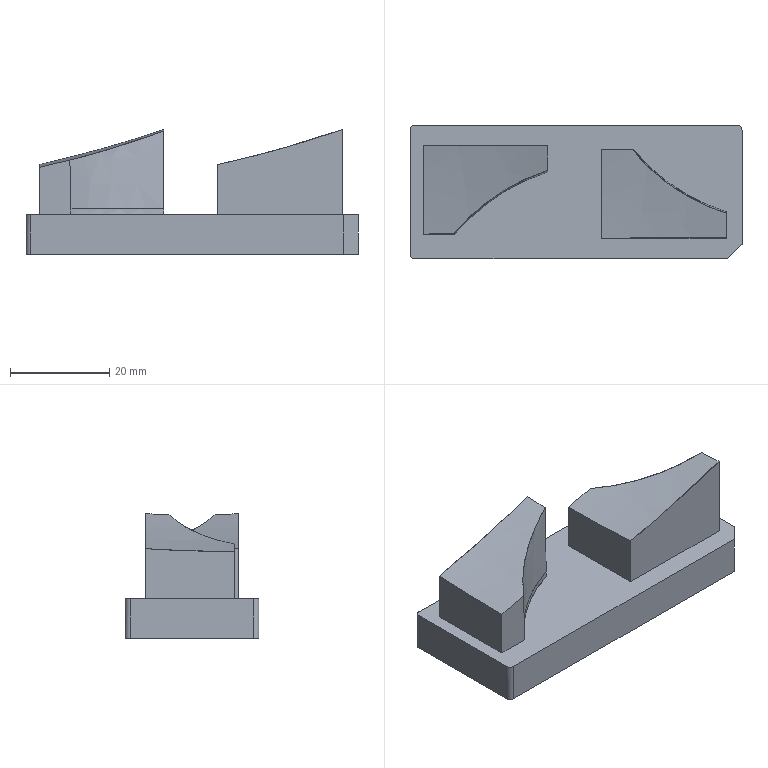NC program | PowerMill | posted with a generic post | part box 67 x 27 x 25.167 mm
Lines 23689 to 24650 of 102458:
N23786 M6
N23787 S8500 M03
N23788 G00 G90 X0.0 Y0.0
N23789 G43 Z9.797 H3
N23790
N23791 G05 P10000 R8
N23792 X40.135 Y-19.0745
N23793 Z-16.17
N23794 G01 Z-17.37 F360.0
N23795 X36.4057 Y-15.3439 F600.0
N23796 X34.1689 Y-13.0592
N23797 X33.9773 Y-13.2468
N23798 X33.7749 Y-13.426
N23799 X33.5166 Y-13.6303
N23800 X33.2073 Y-13.8435
N23801 X32.9235 Y-14.013
N23802 X32.6397 Y-14.1598
N23803 X32.3833 Y-14.2749
N23804 X32.072 Y-14.3937
N23805 X31.7882 Y-14.4832
N23806 X31.5044 Y-14.5561
N23807 X31.2205 Y-14.6127
N23808 X30.9367 Y-14.6536
N23809 X30.6529 Y-14.6795
N23810 X30.3691 Y-14.6899
N23811 X5.3926 Y-14.6902
N23812 X4.825 Y-14.6803
N23813 X4.5412 Y-14.6555
N23814 X4.2573 Y-14.615
N23815 X3.9735 Y-14.5593
N23816 X3.6897 Y-14.4873
N23817 X3.3369 Y-14.3742
N23818 X3.1221 Y-14.2922
N23819 X2.8382 Y-14.1666
N23820 X2.5544 Y-14.0208
N23821 X2.2052 Y-13.8105
N23822 X1.9868 Y-13.6597
N23823 X1.7365 Y-13.4659
N23824 X1.4862 Y-13.2468
N23825 X1.4191 Y-13.1832
N23826 X1.176 Y-12.9332
N23827 X0.9621 Y-12.6831
N23828 X0.8515 Y-12.5408
N23829 X0.7008 Y-12.3301
N23830 X0.5652 Y-12.1194
N23831 X0.4151 Y-11.8584
N23832 X0.2644 Y-11.5557
N23833 X0.1445 Y-11.2739
N23834 X0.0444 Y-10.996
N23835 X-4.5359 Y-12.4333
N23836 X-4.3358 Y-13.0709
N23837 G02 X-5.147 Y-14.1735 I-0.8096 J-0.2541
N23838 G01 X-14.377 Y-14.1571
N23839 G02 X-14.741 Y-13.0303 I0.0011 J0.6226
N23840 G01 X-10.5969 Y-10.0346
N23841 X-6.3435 Y-7.1501
N23842 G02 X-5.0758 Y-7.797 I0.4556 J-0.6727
N23843 G01 X-4.996 Y-10.0671
N23844 X-4.9702 Y-10.3568
N23845 G03 X-4.5645 Y-12.3422 I9.8507 J0.9785
N23846 G01 X-4.5359 Y-12.4333
N23847 X0.0444 Y-10.996
N23848 X-0.0412 Y-10.7102
N23849 X-0.1092 Y-10.4283
N23850 X-0.1613 Y-10.1465
N23851 X-0.1979 Y-9.8647
N23852 X-0.2197 Y-9.5828
N23853 X-0.2267 Y-9.301
N23854 Y8.1736
N23855 X-0.2215 Y8.7373
N23856 X-0.2016 Y9.0191
N23857 X-0.1666 Y9.301
N23858 X-0.1165 Y9.5828
N23859 X-0.0507 Y9.8647
N23860 X0.0314 Y10.1465
N23861 X0.1308 Y10.4283
N23862 X0.2838 Y10.7873
N23863 X0.3853 Y10.992
N23864 X0.5437 Y11.2739
N23865 X0.7254 Y11.5557
N23866 X0.8515 Y11.7308
N23867 X1.0044 Y11.9251
N23868 X1.173 Y12.1194
N23869 X1.4191 Y12.3729
N23870 X1.5947 Y12.5349
N23871 X1.7703 Y12.6831
N23872 X1.9868 Y12.8494
N23873 X2.2706 Y13.0424
N23874 X2.6212 Y13.2468
N23875 X2.8716 Y13.3726
N23876 X3.1221 Y13.4819
N23877 X3.4059 Y13.5884
N23878 X3.6897 Y13.6773
N23879 X3.9735 Y13.7491
N23880 X4.2914 Y13.8105
N23881 X4.5582 Y13.8472
N23882 X4.825 Y13.87
N23883 X5.3926 Y13.8801
N23884 X11.6367 Y13.8799
N23885 X11.9206 Y13.8694
N23886 X12.2044 Y13.8435
N23887 X12.4408 Y13.8105
N23888 X12.772 Y13.7461
N23889 X13.0559 Y13.6733
N23890 X13.3397 Y13.5837
N23891 X13.6235 Y13.4765
N23892 X13.9073 Y13.35
N23893 X14.1111 Y13.2468
N23894 X14.475 Y13.0341
N23895 X14.7186 Y12.8691
N23896 X14.9622 Y12.6831
N23897 X15.0426 Y12.6168
N23898 X15.3011 Y12.3847
N23899 X15.5595 Y12.1194
N23900 X16.1779 Y11.3986
N23901 X16.7456 Y10.763
N23902 X17.0693 Y10.4137
N23903 X17.3978 Y10.0689
N23904 X21.1339 Y13.141
N23905 G02 X21.6149 Y14.1556 I0.4792 J0.3941
N23906 G01 X31.6822 Y14.1268
N23907 G02 X34.0945 Y11.7347 I-0.0069 J-2.4194
N23908 G01 X34.1515 Y6.6925
N23909 G02 X32.8059 Y5.8716 I-0.9169 J-0.0104
N23910 G01 X28.5957 Y8.0987
N23911 G02 X25.0792 Y10.2788 I14.1513 J26.7526
N23912 G01 X21.2509 Y13.0313
N23913 G02 X21.1339 Y13.141 I0.3622 J0.5038
N23914 G01 X17.3978 Y10.0689
N23915 G03 X19.5838 Y7.9955 I24.7883 J23.9452
N23916 G01 X20.1514 Y7.5122
N23917 X20.7191 Y7.0503
N23918 X21.2867 Y6.6069
N23919 G03 X22.422 Y5.7762 I22.7201 J29.8605
N23920 G01 X23.036 Y5.3551
N23921 X23.5573 Y5.0143
N23922 X24.125 Y4.6576
N23923 X24.8412 Y4.2277
N23924 X25.2603 Y3.9882
N23925 X25.847 Y3.664
N23926 X26.3955 Y3.3736
N23927 X26.9363 Y3.1003
N23928 X27.5308 Y2.8143
N23929 X28.1365 Y2.5366
N23930 X28.6661 Y2.3054
N23931 X29.2338 Y2.0682
N23932 X29.8014 Y1.8433
N23933 X30.3691 Y1.63
N23934 X30.9905 Y1.4092
N23935 X32.072 Y1.0514
N23936 X32.3263 Y0.9563
N23937 X32.6397 Y0.8177
N23938 X32.9235 Y0.6709
N23939 X33.2073 Y0.5015
N23940 X33.5252 Y0.2818
N23941 X33.7749 Y0.0839
N23942 X33.9715 Y-0.0895
N23943 X34.168 Y-0.2818
N23944 X34.3426 Y-0.4704
N23945 X34.5009 Y-0.658
N23946 X34.6453 Y-0.8455
N23947 X34.784 Y-1.0437
N23948 X34.9102 Y-1.2419
N23949 X35.0078 Y-1.4092
N23950 X35.1543 Y-1.6911
N23951 X35.2808 Y-1.9729
N23952 X35.388 Y-2.2542
N23953 X35.4784 Y-2.5366
N23954 X35.5515 Y-2.8185
N23955 X35.609 Y-3.1003
N23956 X35.6508 Y-3.3822
N23957 X35.6777 Y-3.664
N23958 X35.6897 Y-3.9459
N23959 X35.6905 Y-9.301
N23960 X35.6833 Y-9.5828
N23961 X35.6616 Y-9.8647
N23962 X35.6249 Y-10.1465
N23963 X35.5727 Y-10.4283
N23964 X35.4779 Y-10.8065
N23965 X35.4205 Y-10.992
N23966 X35.319 Y-11.2739
N23967 X35.1993 Y-11.5557
N23968 X35.0647 Y-11.8279
N23969 X34.8986 Y-12.1194
N23970 X34.7137 Y-12.4013
N23971 X34.5017 Y-12.6831
N23972 X34.3426 Y-12.8717
N23973 X34.1689 Y-13.0592
N23974 X36.4057 Y-15.3439
N23975 G00 Z2.8565
N23976 G01 X-44.255 Y-9.0749 F10000.0
N23977 G00 Z-16.17
N23978 G01 Z-17.37 F360.0
N23979 X-38.98 F600.0
N23980 X-36.2115 Y-8.8782
N23981 X-36.2215 Y-8.7373
N23982 X-36.2265 Y-8.1736
N23983 Y9.301
N23984 X-36.2198 Y9.5828
N23985 X-36.198 Y9.8647
N23986 X-36.1611 Y10.1465
N23987 X-36.1093 Y10.4283
N23988 X-36.0455 Y10.694
N23989 X-35.9571 Y10.992
N23990 X-35.8555 Y11.2739
N23991 X-35.7357 Y11.5557
N23992 X-35.615 Y11.8018
N23993 X-35.4349 Y12.1194
N23994 X-35.25 Y12.4013
N23995 X-35.038 Y12.6831
N23996 X-34.9102 Y12.8359
N23997 X-34.7225 Y13.0413
N23998 X-34.5136 Y13.2468
N23999 X-34.3426 Y13.3996
N24000 X-34.0687 Y13.6185
N24001 X-33.7749 Y13.8234
N24002 X-33.4911 Y13.9954
N24003 X-33.2073 Y14.1447
N24004 X-32.9353 Y14.2682
N24005 X-32.6397 Y14.3827
N24006 X-32.3558 Y14.4744
N24007 X-32.072 Y14.549
N24008 X-31.7882 Y14.6075
N24009 X-31.5044 Y14.65
N24010 X-31.2205 Y14.6772
N24011 X-30.9367 Y14.6896
N24012 X-5.9603 Y14.6902
N24013 X-5.3926 Y14.6822
N24014 X-5.1088 Y14.6589
N24015 X-4.825 Y14.6203
N24016 X-4.5412 Y14.5663
N24017 X-4.2573 Y14.4961
N24018 X-3.8732 Y14.3742
N24019 X-3.6897 Y14.3046
N24020 X-3.4059 Y14.1814
N24021 X-3.1221 Y14.0379
N24022 X-2.9318 Y13.9298
N24023 X-2.7415 Y13.8105
N24024 X-2.5544 Y13.6822
N24025 X-2.2886 Y13.4789
N24026 X-1.9868 Y13.213
N24027 X-1.726 Y12.948
N24028 X-1.4984 Y12.6831
N24029 X-1.4191 Y12.5821
N24030 X-1.2514 Y12.3508
N24031 X-1.1015 Y12.1194
N24032 X-0.9693 Y11.8911
N24033 X-0.8515 Y11.6628
N24034 X-0.8007 Y11.5557
N24035 X-0.6809 Y11.2739
N24036 X-0.5793 Y10.992
N24037 X-0.495 Y10.7102
N24038 X-0.4271 Y10.4283
N24039 X-0.3751 Y10.1465
N24040 X-0.3384 Y9.8647
N24041 X-0.3167 Y9.5828
N24042 X-0.3096 Y9.301
N24043 X-0.3105 Y3.9459
N24044 X-0.3223 Y3.664
N24045 X-0.3492 Y3.3822
N24046 X-0.3911 Y3.1003
N24047 X-0.4483 Y2.8185
N24048 X-0.5216 Y2.5366
N24049 X-0.6117 Y2.2548
N24050 X-0.7193 Y1.9729
N24051 X-0.8515 Y1.6792
N24052 X-0.9923 Y1.4092
N24053 X-1.1611 Y1.1274
N24054 X-1.3548 Y0.8455
N24055 X-1.4191 Y0.7599
N24056 X-1.6132 Y0.5209
N24057 X-1.8321 Y0.2818
N24058 X-1.9868 Y0.1291
N24059 X-2.2308 Y-0.0887
N24060 X-2.4749 Y-0.2818
N24061 X-2.5544 Y-0.3402
N24062 X-2.8382 Y-0.5305
N24063 X-3.1221 Y-0.6958
N24064 X-3.4192 Y-0.8455
N24065 X-3.6897 Y-0.9625
N24066 X-3.9735 Y-1.0672
N24067 X-4.825 Y-1.3454
N24068 X-5.3926 Y-1.5433
N24069 X-5.9603 Y-1.7527
N24070 X-6.5279 Y-1.9729
N24071 X-7.0956 Y-2.2041
N24072 G03 X-8.2309 Y-2.7029 I14.2852 J-34.0594
N24073 G01 X-9.0834 Y-3.1103
N24074 X-9.9338 Y-3.547
N24075 X-10.5015 Y-3.8542
N24076 X-11.0691 Y-4.1757
N24077 G03 X-12.0899 Y-4.7914 I17.2458 J-29.7466
N24078 G01 X-12.9638 Y-5.3551
N24079 X-13.4378 Y-5.68
N24080 X-13.9073 Y-6.0113
N24081 X-14.5476 Y-6.4825
N24082 X-15.0426 Y-6.8623
N24083 G03 X-16.1779 Y-7.7899 I20.6663 J-26.4532
N24084 G01 X-16.6208 Y-8.1736
N24085 X-17.3132 Y-8.8028
N24086 X-17.8809 Y-9.3444
N24087 X-18.4485 Y-9.9114
N24088 X-19.0161 Y-10.506
N24089 X-19.5838 Y-11.1294
N24090 X-20.1514 Y-11.7845
N24091 X-20.4405 Y-12.1194
N24092 X-20.5772 Y-12.2642
N24093 X-20.7191 Y-12.4038
N24094 X-20.8785 Y-12.5489
N24095 X-21.0378 Y-12.6831
N24096 X-21.2867 Y-12.8728
N24097 X-21.5706 Y-13.0627
N24098 X-21.8887 Y-13.2468
N24099 X-22.1554 Y-13.3797
N24100 X-22.422 Y-13.4948
N24101 X-22.7058 Y-13.5993
N24102 X-22.9897 Y-13.6861
N24103 X-23.2735 Y-13.7562
N24104 X-23.5573 Y-13.8102
N24105 X-23.8421 Y-13.8488
N24106 X-24.125 Y-13.8719
N24107 X-24.6926 Y-13.8801
N24108 X-30.9367 Y-13.8793
N24109 X-31.2205 Y-13.8671
N24110 X-31.5044 Y-13.8397
N24111 X-31.7086 Y-13.8105
N24112 X-32.072 Y-13.7387
N24113 X-32.3558 Y-13.6642
N24114 X-32.6397 Y-13.5724
N24115 X-32.9235 Y-13.4631
N24116 X-33.2073 Y-13.3346
N24117 X-33.3789 Y-13.2468
N24118 X-33.5769 Y-13.1357
N24119 X-33.7749 Y-13.0134
N24120 X-34.0024 Y-12.8574
N24121 X-34.2298 Y-12.6831
N24122 X-34.3426 Y-12.5893
N24123 X-34.5848 Y-12.3693
N24124 X-34.8271 Y-12.1194
N24125 X-34.9102 Y-12.0258
N24126 X-35.1028 Y-11.7908
N24127 X-35.2747 Y-11.5557
N24128 X-35.4779 Y-11.2378
N24129 X-35.6148 Y-10.992
N24130 X-35.7518 Y-10.7102
N24131 X-35.8692 Y-10.4283
N24132 X-35.9655 Y-10.1561
N24133 X-36.0508 Y-9.8647
N24134 X-36.1166 Y-9.5828
N24135 X-36.1667 Y-9.301
N24136 X-36.2015 Y-9.0191
N24137 X-36.2115 Y-8.8782
N24138 X-38.98 Y-9.0749
N24139 G00 Z9.797
N24140 G05 P0
N24141 (---------------)
N24142 ( END TOOLPATH : 精公基准台01-基准面偏置-D10 )
N24143 (---------------)
N24144 ( START TOOLPATH : 精公基准台01-外形侧光-D10 )
N24145 (---------------)
N24146 G00 X0.0 Y0.0 Z10.797
N24147 G05 P10000 R8
N24148 X34.6648 Y-12.7529
N24149 Z-16.14
N24150 G01 Z-17.34 F360.0
N24151 G03 X33.5738 Y-13.1106 I-0.1138 J-1.4957 F600.0
N24152 G02 X30.3043 Y-14.3202 I-3.2654 J3.803
N24153 G01 X17.9818 Y-14.3201
N24154 X5.1094 Y-14.32
N24155 G02 X0.1435 Y-9.2191 I0.0459 J5.0124
N24156 G01 Y8.4902
N24157 G02 X5.1116 Y13.5098 I5.01 J0.0097
N24158 G01 X11.5015 Y13.51
N24159 G02 X15.3956 Y11.7453 I0.0742 J-5.0152
N24160 G03 X31.7901 Y0.7551 I26.8851 J22.3821
N24161 G02 X35.3201 Y-4.1075 I-1.4846 J-4.7904
N24162 G01 Y-9.2195
N24163 G02 X33.5738 Y-13.1106 I-5.0117 J-0.0881
N24164 G03 X33.0554 Y-14.1349 I0.9773 J-1.138
N24165 G01 X34.6023 Y-12.7054
N24166 G03 X33.5103 Y-13.0597 I-0.1183 J-1.4953
N24167 G02 X30.3043 Y-14.2402 I-3.2019 J3.7521
N24168 G01 X17.9818
N24169 X5.1116 Y-14.24
N24170 G02 X0.2235 Y-9.2191 I0.0437 J4.9324
N24171 G01 Y8.4889
N24172 G02 X5.1116 Y13.4298 I4.93 J0.0111
N24173 G01 X11.501 Y13.43
N24174 G02 X15.3347 Y11.6934 I0.0747 J-4.9351
N24175 G03 X31.7648 Y0.6792 I26.9457 J22.4336
N24176 G02 X35.2401 Y-4.1075 I-1.4593 J-4.7145
N24177 G01 Y-9.2191
N24178 G02 X33.5103 Y-13.0597 I-4.9317 J-0.0885
N24179 G03 X32.9887 Y-14.0824 I0.9737 J-1.141
N24180 G00 Z3.9761
N24181 G01 X-11.096 Y-4.2525 F10000.0
N24182 G00 Z-16.14
N24183 G01 Z-17.34 F360.0
N24184 G03 X-12.2285 Y-4.4408 I-0.339 J-1.4612 F600.0
N24185 G03 X-20.0224 Y-11.066 I18.4655 J-29.6201
N24186 G03 X-20.6769 Y-11.8287 I60.5942 J-52.6567
N24187 G02 X-24.4625 Y-13.51 I-3.7452 J3.3303
N24188 G01 X-30.8536
N24189 G02 X-35.8565 Y-8.4889 I0.0071 J5.0101
N24190 G01 Y9.2195
N24191 G02 X-30.852 Y14.3202 I5.0117 J0.0881
N24192 G01 X-5.6573 Y14.3201
N24193 G02 X-0.6799 Y9.2191 I-0.0344 J-5.0125
N24194 G01 Y4.107
N24195 G02 X-1.725 Y0.9692 I-5.0182 J-0.0714
N24196 G02 X-1.7373 Y0.9534 I-3.9601 J3.0563
N24197 G02 X-4.0877 Y-0.715 I-3.9525 J3.0784
N24198 G03 X-6.3604 Y-1.509 I11.0352 J-35.2381
N24199 G03 X-12.2285 Y-4.4408 I12.5975 J-32.5519
N24200 G03 X-12.8962 Y-5.3748 I0.7935 J-1.2729
N24201 G01 X-11.1618 Y-4.1993
N24202 G03 X-12.2941 Y-4.3886 I-0.3377 J-1.4615
N24203 G03 X-20.0825 Y-11.0132 I18.5558 J-29.7062
N24204 G03 X-20.7361 Y-11.7749 I60.0264 J-52.1654
N24205 G02 X-24.4625 Y-13.43 I-3.686 J3.2764
N24206 G01 X-30.852
N24207 G02 X-35.7765 Y-8.4889 I0.0055 J4.93
N24208 G01 Y9.2191
N24209 G02 X-30.852 Y14.2402 I4.9317 J0.0885
N24210 G01 X-5.6592 Y14.2401
N24211 G02 X-0.7599 Y9.2191 I-0.0325 J-4.9325
N24212 G01 Y4.1075
N24213 G02 X-1.7883 Y1.0181 I-4.9384 J-0.0719
N24214 G02 X-1.7992 Y1.0041 I-3.8737 J2.9895
N24215 G02 X-4.1125 Y-0.6389 I-3.8907 J3.0278
N24216 G01 X-4.929 Y-0.9052
N24217 G03 X-12.2941 Y-4.3886 I11.1907 J-33.1896
N24218 G03 X-12.961 Y-5.3231 I0.7946 J-1.2722
N24219 G00 Z10.797
N24220 G05 P0
N24221 (---------------)
N24222 ( END TOOLPATH : 精公基准台01-外形侧光-D10 )
N24223 (---------------)
N24224 ( START TOOLPATH : 精公基准台01-基准台侧光-D10 )
N24225 (---------------)
N24226 G00 X0.0 Y0.0 Z9.797
N24227 G05 P10000 R8
N24228 X38.3252 Y-19.9298
N24229 Z-24.07
N24230 G01 Z-25.27 F360.0
N24231 G03 X34.7899 Y-16.394 I-1.7677 J1.7679 F600.0
N24232 G01 X34.0554 Y-17.1284
N24233 X34.0544 Y-17.1294
N24234 X34.0535 Y-17.1303
N24235 X33.8822 Y-17.2904
N24236 X33.8808 Y-17.2916
N24237 X33.8794 Y-17.2929
N24238 X33.6956 Y-17.449
N24239 X33.6943 Y-17.45
N24240 X33.693 Y-17.4511
N24241 X33.5607 Y-17.5545
N24242 X33.559 Y-17.5558
N24243 X33.5572 Y-17.557
N24244 X33.2523 Y-17.7698
N24245 X33.2498 Y-17.7714
N24246 X33.2472 Y-17.773
N24247 X32.9199 Y-17.9666
N24248 X32.9173 Y-17.968
N24249 X32.9147 Y-17.9694
N24250 X32.5986 Y-18.1262
N24251 X32.5961 Y-18.1274
N24252 X32.5935 Y-18.1285
N24253 X32.2774 Y-18.2589
N24254 X32.2748 Y-18.2599
N24255 X32.2723 Y-18.2608
N24256 X31.9561 Y-18.3668
N24257 X31.9542 Y-18.3674
N24258 X31.9523 Y-18.368
N24259 X31.79 Y-18.4135
N24260 X31.7887 Y-18.4138
N24261 X31.7874 Y-18.4141
N24262 X31.6336 Y-18.4519
N24263 X31.6318 Y-18.4523
N24264 X31.6299 Y-18.4527
N24265 X31.3137 Y-18.5144
N24266 X31.3112 Y-18.5148
N24267 X31.3087 Y-18.5152
N24268 X30.9925 Y-18.556
N24269 X30.99 Y-18.5563
N24270 X30.9875 Y-18.5565
N24271 X30.6713 Y-18.5771
N24272 X30.6691 Y-18.5772
N24273 X30.6668
N24274 X30.3507 Y-18.58
N24275 X30.3503
N24276 X30.35
N24277 X-32.563 Y-18.5796
N24278 X-32.5645
N24279 X-32.5659
N24280 X-32.8821 Y-18.568
N24281 X-32.8842 Y-18.5679
N24282 X-32.8863 Y-18.5677
N24283 X-33.2025 Y-18.5392
N24284 X-33.2046 Y-18.539
N24285 X-33.2067 Y-18.5387
N24286 X-33.5228 Y-18.4933
N24287 X-33.5249 Y-18.493
N24288 X-33.5271 Y-18.4926
N24289 X-33.8432 Y-18.4297
N24290 X-33.8453 Y-18.4292
N24291 X-33.8474 Y-18.4287
N24292 X-34.1636 Y-18.3478
N24293 X-34.1657 Y-18.3473
N24294 X-34.1678 Y-18.3466
N24295 X-34.4839 Y-18.2471
N24296 X-34.486 Y-18.2464
N24297 X-34.4881 Y-18.2456
N24298 X-34.8043 Y-18.1264
N24299 X-34.8064 Y-18.1256
N24300 X-34.8085 Y-18.1247
N24301 X-35.1247 Y-17.9842
N24302 X-35.1268 Y-17.9832
N24303 X-35.1289 Y-17.9821
N24304 X-35.445 Y-17.8189
N24305 X-35.4471 Y-17.8178
N24306 X-35.4492 Y-17.8166
N24307 X-35.7654 Y-17.6285
N24308 X-35.7675 Y-17.6272
N24309 X-35.7696 Y-17.6258
N24310 X-36.0857 Y-17.41
N24311 X-36.0879 Y-17.4085
N24312 X-36.09 Y-17.4069
N24313 X-36.4061 Y-17.1592
N24314 X-36.4082 Y-17.1575
N24315 X-36.4103 Y-17.1557
N24316 X-36.7265 Y-16.8706
N24317 X-36.7277 Y-16.8695
N24318 X-36.7289 Y-16.8683
N24319 X-36.7855 Y-16.8129
N24320 X-36.7866 Y-16.8118
N24321 X-36.7877 Y-16.8107
N24322 X-37.0472 Y-16.5359
N24323 X-37.0491 Y-16.5338
N24324 X-37.0509 Y-16.5317
N24325 X-37.3442 Y-16.1742
N24326 X-37.346 Y-16.1719
N24327 X-37.3477 Y-16.1695
N24328 X-37.5707 Y-15.8534
N24329 X-37.5717 Y-15.8519
N24330 X-37.5727 Y-15.8504
N24331 X-37.6887 Y-15.6691
N24332 X-37.6894 Y-15.668
N24333 X-37.6902 Y-15.6668
N24334 X-37.7701 Y-15.5319
N24335 X-37.7709 Y-15.5304
N24336 X-37.7718 Y-15.5289
N24337 X-37.9412 Y-15.2128
N24338 X-37.942 Y-15.2113
N24339 X-37.9428 Y-15.2097
N24340 X-38.0095 Y-15.0712
N24341 X-38.01 Y-15.0702
N24342 X-38.0105 Y-15.0691
N24343 X-38.0899 Y-14.8915
N24344 X-38.0906 Y-14.8898
N24345 X-38.0912 Y-14.8882
N24346 X-38.216 Y-14.5721
N24347 X-38.2168 Y-14.57
N24348 X-38.2175 Y-14.5678
N24349 X-38.3222 Y-14.2517
N24350 X-38.3228 Y-14.2496
N24351 X-38.3234 Y-14.2475
N24352 X-38.4091 Y-13.9313
N24353 X-38.4096 Y-13.9292
N24354 X-38.4101 Y-13.927
N24355 X-38.4772 Y-13.6109
N24356 X-38.4776 Y-13.6089
N24357 X-38.478 Y-13.6069
N24358 X-38.5283 Y-13.2907
N24359 X-38.5287 Y-13.2885
N24360 X-38.5289 Y-13.2863
N24361 X-38.5614 Y-12.9701
N24362 X-38.5616 Y-12.9681
N24363 X-38.5617 Y-12.966
N24364 X-38.5778 Y-12.6499
N24365 Y-12.6481
N24366 X-38.5779 Y-12.6464
N24367 X-38.58 Y-12.3302
N24368 Y-12.3299
N24369 Y-12.3297
N24370 Y12.3297
N24371 Y12.3299
N24372 Y12.3302
N24373 X-38.5779 Y12.6464
N24374 X-38.5778 Y12.6481
N24375 Y12.6498
N24376 X-38.5621 Y12.9659
N24377 X-38.562 Y12.9681
N24378 X-38.5618 Y12.9702
N24379 X-38.5289 Y13.2864
N24380 X-38.5287 Y13.2885
N24381 X-38.5284 Y13.2906
N24382 X-38.4784 Y13.6068
N24383 X-38.478 Y13.6089
N24384 X-38.4776 Y13.611
N24385 X-38.4101 Y13.9271
N24386 X-38.4096 Y13.9291
N24387 X-38.4091 Y13.9312
N24388 X-38.3309 Y14.2224
N24389 X-38.3303 Y14.2245
N24390 X-38.3296 Y14.2267
N24391 X-38.2171 Y14.5678
N24392 X-38.2164 Y14.5699
N24393 X-38.2156 Y14.572
N24394 X-38.0913 Y14.8881
N24395 X-38.0906 Y14.8898
N24396 X-38.0899 Y14.8915
N24397 X-38.0105 Y15.0691
N24398 X-38.01 Y15.0703
N24399 X-38.0094 Y15.0715
N24400 X-37.9421 Y15.21
N24401 X-37.9414 Y15.2113
N24402 X-37.9407 Y15.2127
N24403 X-37.7718 Y15.5288
N24404 X-37.771 Y15.5304
N24405 X-37.7701 Y15.5319
N24406 X-37.6902 Y15.6668
N24407 X-37.6895 Y15.6679
N24408 X-37.6889 Y15.6689
N24409 X-37.5737 Y15.8502
N24410 X-37.5727 Y15.8518
N24411 X-37.5716 Y15.8533
N24412 X-37.3706 Y16.139
N24413 X-37.3691 Y16.1411
N24414 X-37.3674 Y16.1432
N24415 X-37.0877 Y16.4898
N24416 X-37.0858 Y16.4921
N24417 X-37.0839 Y16.4942
N24418 X-36.7879 Y16.8104
N24419 X-36.7867 Y16.8117
N24420 X-36.7854 Y16.8129
N24421 X-36.7288 Y16.8683
N24422 X-36.7277 Y16.8693
N24423 X-36.7266 Y16.8704
N24424 X-36.4386 Y17.1312
N24425 X-36.4365 Y17.1329
N24426 X-36.4345 Y17.1346
N24427 X-36.0902 Y17.4067
N24428 X-36.088 Y17.4084
N24429 X-36.0857 Y17.41
N24430 X-35.7696 Y17.6258
N24431 X-35.7678 Y17.627
N24432 X-35.7659 Y17.6281
N24433 X-35.5275 Y17.7726
N24434 X-35.5254 Y17.7738
N24435 X-35.5233 Y17.775
N24436 X-35.1294 Y17.982
N24437 X-35.1273 Y17.9831
N24438 X-35.1251 Y17.9841
N24439 X-34.8836 Y18.0932
N24440 X-34.8815 Y18.0941
N24441 X-34.8794 Y18.095
N24442 X-34.4886 Y18.2455
N24443 X-34.4863 Y18.2464
N24444 X-34.4839 Y18.2472
N24445 X-34.1677 Y18.3467
N24446 X-34.1659 Y18.3473
N24447 X-34.164 Y18.3478
N24448 X-33.9116 Y18.4138
N24449 X-33.9094 Y18.4144
N24450 X-33.9072 Y18.4149
N24451 X-33.5273 Y18.4918
N24452 X-33.5252 Y18.4922
N24453 X-33.523 Y18.4925
N24454 X-33.2068 Y18.5387
N24455 X-33.2045 Y18.539
N24456 X-33.2022 Y18.5392
N24457 X-32.8861 Y18.5668
N24458 X-32.8842 Y18.5669
N24459 X-32.8823 Y18.567
N24460 X-32.5662 Y18.5795
N24461 X-32.5646 Y18.5796
N24462 X-32.563
N24463 X0.0
N24464 X32.563
N24465 X32.5645
N24466 X32.5659 Y18.5795
N24467 X32.8821 Y18.568
N24468 X32.8842 Y18.5679
N24469 X32.8863 Y18.5677
N24470 X33.2025 Y18.5392
N24471 X33.2046 Y18.539
N24472 X33.2067 Y18.5387
N24473 X33.5228 Y18.4933
N24474 X33.5249 Y18.493
N24475 X33.5271 Y18.4926
N24476 X33.8432 Y18.4297
N24477 X33.8453 Y18.4292
N24478 X33.8474 Y18.4287
N24479 X34.1636 Y18.3478
N24480 X34.1657 Y18.3473
N24481 X34.1678 Y18.3466
N24482 X34.4839 Y18.2471
N24483 X34.486 Y18.2464
N24484 X34.4881 Y18.2456
N24485 X34.8043 Y18.1264
N24486 X34.8064 Y18.1256
N24487 X34.8085 Y18.1246
N24488 X35.1247 Y17.9842
N24489 X35.1268 Y17.9832
N24490 X35.1289 Y17.9821
N24491 X35.445 Y17.8189
N24492 X35.4471 Y17.8178
N24493 X35.4492 Y17.8166
N24494 X35.7654 Y17.6285
N24495 X35.7675 Y17.6272
N24496 X35.7696 Y17.6258
N24497 X36.0857 Y17.41
N24498 X36.0879 Y17.4085
N24499 X36.09 Y17.4069
N24500 X36.4061 Y17.1592
N24501 X36.4082 Y17.1575
N24502 X36.4103 Y17.1557
N24503 X36.7265 Y16.8706
N24504 X36.7277 Y16.8695
N24505 X36.7289 Y16.8683
N24506 X36.7855 Y16.8129
N24507 X36.7866 Y16.8118
N24508 X36.7877 Y16.8107
N24509 X37.0472 Y16.5359
N24510 X37.0491 Y16.5338
N24511 X37.0509 Y16.5317
N24512 X37.3442 Y16.1742
N24513 X37.346 Y16.1719
N24514 X37.3477 Y16.1695
N24515 X37.5707 Y15.8534
N24516 X37.5717 Y15.8519
N24517 X37.5727 Y15.8504
N24518 X37.6887 Y15.6691
N24519 X37.6894 Y15.668
N24520 X37.6902 Y15.6668
N24521 X37.7701 Y15.5319
N24522 X37.7709 Y15.5304
N24523 X37.7718 Y15.5289
N24524 X37.9412 Y15.2128
N24525 X37.942 Y15.2113
N24526 X37.9428 Y15.2097
N24527 X38.0095 Y15.0712
N24528 X38.01 Y15.0702
N24529 X38.0105 Y15.0691
N24530 X38.0899 Y14.8915
N24531 X38.0906 Y14.8898
N24532 X38.0912 Y14.8882
N24533 X38.216 Y14.5721
N24534 X38.2168 Y14.57
N24535 X38.2175 Y14.5678
N24536 X38.3222 Y14.2517
N24537 X38.3228 Y14.2496
N24538 X38.3234 Y14.2475
N24539 X38.4091 Y13.9313
N24540 X38.4096 Y13.9292
N24541 X38.4101 Y13.927
N24542 X38.4772 Y13.6109
N24543 X38.4776 Y13.6089
N24544 X38.478 Y13.6069
N24545 X38.5283 Y13.2907
N24546 X38.5287 Y13.2885
N24547 X38.5289 Y13.2863
N24548 X38.5614 Y12.9701
N24549 X38.5616 Y12.9681
N24550 X38.5617 Y12.966
N24551 X38.5778 Y12.6499
N24552 X38.5779 Y12.6481
N24553 Y12.6464
N24554 X38.58 Y12.3302
N24555 Y12.3299
N24556 Y12.3297
N24557 Y-10.4328
N24558 Y-10.4336
N24559 Y-10.4344
N24560 X38.5738 Y-10.7505
N24561 X38.5737 Y-10.753
N24562 X38.5735 Y-10.7555
N24563 X38.5477 Y-11.0716
N24564 X38.5475 Y-11.0741
N24565 X38.5471 Y-11.0767
N24566 X38.5009 Y-11.3928
N24567 X38.5005 Y-11.3954
N24568 X38.5 Y-11.3979
N24569 X38.4328 Y-11.714
N24570 X38.4322 Y-11.7166
N24571 X38.4315 Y-11.7191
N24572 X38.3424 Y-12.0352
N24573 X38.3417 Y-12.0378
N24574 X38.3408 Y-12.0403
N24575 X38.2286 Y-12.3564
N24576 X38.2276 Y-12.359
N24577 X38.2266 Y-12.3615
N24578 X38.0895 Y-12.6776
N24579 X38.0887 Y-12.6796
N24580 X38.0878 Y-12.6814
N24581 X38.0091 Y-12.8397
N24582 X38.0085 Y-12.841
N24583 X38.0078 Y-12.8422
N24584 X37.9222 Y-13.0001
N24585 X37.9211 Y-13.002
N24586 X37.92 Y-13.0039
N24587 X37.7253 Y-13.3201
N24588 X37.7236 Y-13.3226
N24589 X37.7219 Y-13.3251
N24590 X37.4923 Y-13.6413
N24591 X37.4909 Y-13.6431
N24592 X37.4894 Y-13.645
N24593 X37.3671 Y-13.7943
N24594 X37.366 Y-13.7955
N24595 X37.3649 Y-13.7968
N24596 X37.2161 Y-13.9637
N24597 X37.2149 Y-13.965
N24598 X37.2137 Y-13.9663
N24599 X37.0463 Y-14.1379
N24600 X37.046 Y-14.1382
N24601 X37.0456 Y-14.1386
N24602 X34.7899 Y-16.394
N24603 G03 X38.3252 Y-19.9298 I1.7677 J-1.7679
N24604 G01 X38.275 Y-19.8669
N24605 G03 X34.7397 Y-16.3311 I-1.7677 J1.7679
N24606 G01 X33.9988 Y-17.0719
N24607 X33.8276 Y-17.2319
N24608 X33.6438 Y-17.388
N24609 X33.5114 Y-17.4914
N24610 X33.2065 Y-17.7042
N24611 X32.8792 Y-17.8977
N24612 X32.563 Y-18.0546
N24613 X32.2469 Y-18.1849
N24614 X31.9307 Y-18.2909
N24615 X31.7684 Y-18.3364
N24616 X31.6146 Y-18.3742
N24617 X31.2984 Y-18.4359
N24618 X30.9823 Y-18.4767
N24619 X30.6661 Y-18.4972
N24620 X30.35 Y-18.5
N24621 X-32.563 Y-18.4996
N24622 X-32.8792 Y-18.488
N24623 X-33.1953 Y-18.4595
N24624 X-33.5114 Y-18.4141
N24625 X-33.8276 Y-18.3512
N24626 X-34.1437 Y-18.2703
N24627 X-34.4599 Y-18.1708
N24628 X-34.776 Y-18.0516
N24629 X-35.0922 Y-17.9111
N24630 X-35.4083 Y-17.7478
N24631 X-35.7245 Y-17.5597
N24632 X-36.0406 Y-17.344
N24633 X-36.3568 Y-17.0963
N24634 X-36.6729 Y-16.8112
N24635 X-36.7295 Y-16.7557
N24636 X-36.989 Y-16.481
N24637 X-37.2823 Y-16.1234
N24638 X-37.5054 Y-15.8073
N24639 X-37.6213 Y-15.626
N24640 X-37.7013 Y-15.4911
N24641 X-37.8707 Y-15.175
N24642 X-37.9375 Y-15.0365
N24643 X-38.0168 Y-14.8588
N24644 X-38.1416 Y-14.5427
N24645 X-38.2462 Y-14.2266
N24646 X-38.3318 Y-13.9104
N24647 X-38.399 Y-13.5943
N24648 X-38.4493 Y-13.2781
N24649 X-38.4818 Y-12.962
N24650 X-38.4979 Y-12.6458
N24651 X-38.5 Y-12.3297
N24652 Y12.3297
N24653 X-38.4979 Y12.6458
N24654 X-38.4822 Y12.962
N24655 X-38.4493 Y13.2781
N24656 X-38.3993 Y13.5943
N24657 X-38.3319 Y13.9104
N24658 X-38.2536 Y14.2016
N24659 X-38.1411 Y14.5427
N24660 X-38.0168 Y14.8588
N24661 X-37.9375 Y15.0365
N24662 X-37.8702 Y15.175
N24663 X-37.7013 Y15.4911
N24664 X-37.6213 Y15.626
N24665 X-37.5062 Y15.8073
N24666 X-37.3052 Y16.0929
N24667 X-37.0254 Y16.4396
N24668 X-36.7295 Y16.7557
N24669 X-36.6729 Y16.8111
N24670 X-36.3849 Y17.0719
N24671 X-36.0406 Y17.344
N24672 X-35.7245 Y17.5597
N24673 X-35.4861 Y17.7042
N24674 X-35.0922 Y17.9112
N24675 X-34.8507 Y18.0203
N24676 X-34.4599 Y18.1709
N24677 X-34.1437 Y18.2704
N24678 X-33.8913 Y18.3364
N24679 X-33.5114 Y18.4134
N24680 X-33.1953 Y18.4595
N24681 X-32.8792 Y18.4871
N24682 X-32.563 Y18.4996
N24683 X0.0
N24684 X32.563
N24685 X32.8792 Y18.488
N24686 X33.1953 Y18.4595
N24687 X33.5114 Y18.4141
N24688 X33.8276 Y18.3512
N24689 X34.1437 Y18.2703
N24690 X34.4599 Y18.1708
N24691 X34.776 Y18.0515
N24692 X35.0922 Y17.9111
N24693 X35.4083 Y17.7478
N24694 X35.7245 Y17.5597
N24695 X36.0406 Y17.344
N24696 X36.3568 Y17.0963
N24697 X36.6729 Y16.8112
N24698 X36.7295 Y16.7557
N24699 X36.989 Y16.481
N24700 X37.2823 Y16.1234
N24701 X37.5054 Y15.8073
N24702 X37.6213 Y15.626
N24703 X37.7013 Y15.4911
N24704 X37.8707 Y15.175
N24705 X37.9375 Y15.0365
N24706 X38.0168 Y14.8588
N24707 X38.1416 Y14.5427
N24708 X38.2462 Y14.2266
N24709 X38.3318 Y13.9104
N24710 X38.399 Y13.5943
N24711 X38.4493 Y13.2781
N24712 X38.4818 Y12.962
N24713 X38.4979 Y12.6458
N24714 X38.5 Y12.3297
N24715 Y-10.4328
N24716 X38.4938 Y-10.749
N24717 X38.468 Y-11.0651
N24718 X38.4217 Y-11.3812
N24719 X38.3545 Y-11.6974
N24720 X38.2654 Y-12.0135
N24721 X38.1532 Y-12.3297
N24722 X38.0161 Y-12.6458
N24723 X37.9375 Y-12.8041
N24724 X37.8519 Y-12.962
N24725 X37.6572 Y-13.2781
N24726 X37.4275 Y-13.5943
N24727 X37.3052 Y-13.7436
N24728 X37.1564 Y-13.9104
N24729 X36.989 Y-14.082
N24730 X34.7397 Y-16.3311
N24731 G03 X38.275 Y-19.8669 I1.7676 J-1.7679
N24732 G00 Z9.797
N24733 G05 P0
N24734 (---------------)
N24735 ( END TOOLPATH : 精公基准台01-基准台侧光-D10 )
N24736 (---------------)
N24737
N24738 M05
N24739 G53 Z0.0
N24740 (---------------)
N24741 ( START TOOLPATH : 精公精光01-平行-R2 )
N24742 (---------------)
N24743 ( TOOL NO.    :7 )
N24744 ( TOOL TYPE   : BALLNOSED)
N24745 ( TOOL ID     : R2_1_1)
N24746 ( TOOL DIA    : 4.0 LENGTH 62.96)
N24747 T7